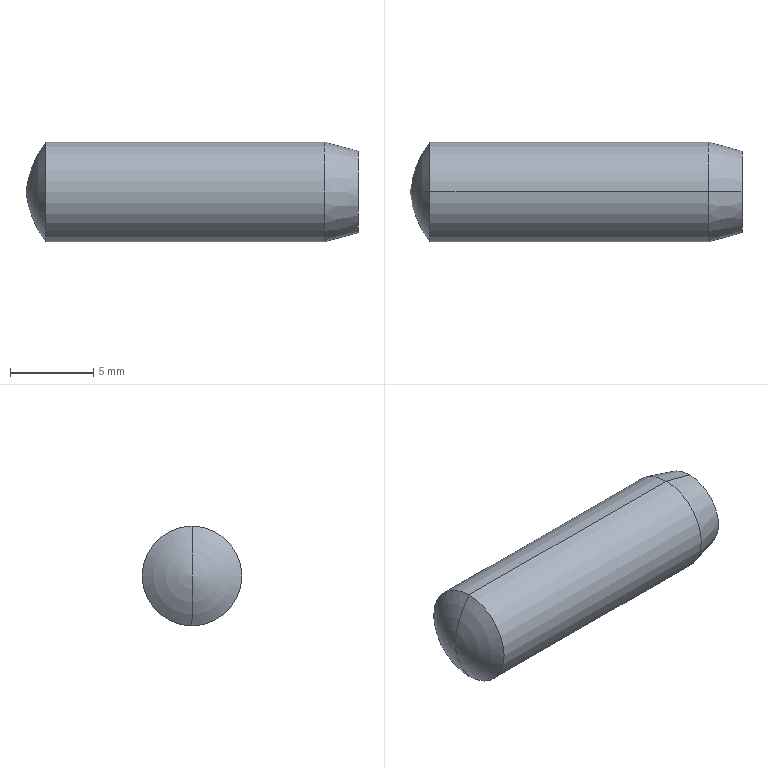Part | SolidWorks | features RefAxis 3, 3DProfileFeature 1, RevCut 1, Revolution 1 | 1 solid | 9 faces | box 20 x 6 x 6 mm | volume 537.381 mm3 | cone 4 | cylinder 2 | torus 2 | plane 1 | commonest cylinder face diameters 6 x2
STEP:
#1=CARTESIAN_POINT('',(8.,0.,0.));
#2=VERTEX_POINT('',#1);
#3=CARTESIAN_POINT('',(10.,0.,-0.5359));
#4=VERTEX_POINT('',#3);
#5=CARTESIAN_POINT('',(12.,0.,-1.072));
#6=DIRECTION('',(0.9659,0.,-0.2588));
#7=VECTOR('',#6,1000.);
#8=LINE('',#5,#7);
#9=EDGE_CURVE('',#2,#4,#8,.T.);
#10=ORIENTED_EDGE('',*,*,#9,.F.);
#11=CARTESIAN_POINT('',(10.,0.,0.5359));
#12=VERTEX_POINT('',#11);
#13=CARTESIAN_POINT('',(12.,0.,1.072));
#14=DIRECTION('',(0.9659,0.,0.2588));
#15=VECTOR('',#14,1000.);
#16=LINE('',#13,#15);
#17=EDGE_CURVE('',#2,#12,#16,.T.);
#18=ORIENTED_EDGE('',*,*,#17,.T.);
#19=CARTESIAN_POINT('',(10.,0.,0.));
#20=DIRECTION('',(1.,0.,0.));
#21=DIRECTION('',(0.,0.,1.));
#22=AXIS2_PLACEMENT_3D('',#19,#20,#21);
#23=CIRCLE('',#22,0.5359);
#24=EDGE_CURVE('',#12,#4,#23,.T.);
#25=ORIENTED_EDGE('',*,*,#24,.T.);
#26=EDGE_LOOP('',(#10,#18,#25));
#27=FACE_OUTER_BOUND('',#26,.T.);
#28=CARTESIAN_POINT('',(12.,0.,0.));
#29=DIRECTION('',(1.,0.,0.));
#30=DIRECTION('',(0.,0.,-1.));
#31=AXIS2_PLACEMENT_3D('',#28,#29,#30);
#32=CONICAL_SURFACE('',#31,1.072,0.2618);
#33=ADVANCED_FACE('',(#27),#32,.F.);
#34=CARTESIAN_POINT('',(10.,0.,2.464));
#35=VERTEX_POINT('',#34);
#36=CARTESIAN_POINT('',(10.,0.,-2.464));
#37=VERTEX_POINT('',#36);
#38=CARTESIAN_POINT('',(10.,0.,0.));
#39=DIRECTION('',(-1.,0.,0.));
#40=DIRECTION('',(0.,0.,1.));
#41=AXIS2_PLACEMENT_3D('',#38,#39,#40);
#42=CIRCLE('',#41,2.464);
#43=EDGE_CURVE('',#35,#37,#42,.T.);
#44=ORIENTED_EDGE('',*,*,#43,.T.);
#45=CARTESIAN_POINT('',(8.,0.,-3.));
#46=VERTEX_POINT('',#45);
#47=CARTESIAN_POINT('',(10.,0.,-2.464));
#48=DIRECTION('',(-0.9659,0.,-0.2588));
#49=VECTOR('',#48,1000.);
#50=LINE('',#47,#49);
#51=EDGE_CURVE('',#37,#46,#50,.T.);
#52=ORIENTED_EDGE('',*,*,#51,.T.);
#53=CARTESIAN_POINT('',(8.,0.,3.));
#54=VERTEX_POINT('',#53);
#55=CARTESIAN_POINT('',(8.,0.,0.));
#56=DIRECTION('',(-1.,0.,0.));
#57=DIRECTION('',(0.,0.,1.));
#58=AXIS2_PLACEMENT_3D('',#55,#56,#57);
#59=CIRCLE('',#58,3.);
#60=EDGE_CURVE('',#54,#46,#59,.T.);
#61=ORIENTED_EDGE('',*,*,#60,.F.);
#62=CARTESIAN_POINT('',(10.,0.,2.464));
#63=DIRECTION('',(-0.9659,0.,0.2588));
#64=VECTOR('',#63,1000.);
#65=LINE('',#62,#64);
#66=EDGE_CURVE('',#35,#54,#65,.T.);
#67=ORIENTED_EDGE('',*,*,#66,.F.);
#68=EDGE_LOOP('',(#44,#52,#61,#67));
#69=FACE_OUTER_BOUND('',#68,.T.);
#70=CARTESIAN_POINT('',(10.,0.,0.));
#71=DIRECTION('',(-1.,0.,0.));
#72=DIRECTION('',(0.,0.,1.));
#73=AXIS2_PLACEMENT_3D('',#70,#71,#72);
#74=CONICAL_SURFACE('',#73,2.464,0.2618);
#75=ADVANCED_FACE('',(#69),#74,.T.);
#76=ORIENTED_EDGE('',*,*,#60,.T.);
#77=CARTESIAN_POINT('',(-8.8,0.,-3.));
#78=VERTEX_POINT('',#77);
#79=CARTESIAN_POINT('',(10.,0.,-3.));
#80=DIRECTION('',(-1.,0.,0.));
#81=VECTOR('',#80,1000.);
#82=LINE('',#79,#81);
#83=EDGE_CURVE('',#46,#78,#82,.T.);
#84=ORIENTED_EDGE('',*,*,#83,.T.);
#85=CARTESIAN_POINT('',(-8.8,0.,3.));
#86=VERTEX_POINT('',#85);
#87=CARTESIAN_POINT('',(-8.8,0.,0.));
#88=DIRECTION('',(-1.,0.,0.));
#89=DIRECTION('',(0.,0.,1.));
#90=AXIS2_PLACEMENT_3D('',#87,#88,#89);
#91=CIRCLE('',#90,3.);
#92=EDGE_CURVE('',#86,#78,#91,.T.);
#93=ORIENTED_EDGE('',*,*,#92,.F.);
#94=CARTESIAN_POINT('',(10.,0.,3.));
#95=DIRECTION('',(-1.,0.,0.));
#96=VECTOR('',#95,1000.);
#97=LINE('',#94,#96);
#98=EDGE_CURVE('',#54,#86,#97,.T.);
#99=ORIENTED_EDGE('',*,*,#98,.F.);
#100=EDGE_LOOP('',(#76,#84,#93,#99));
#101=FACE_OUTER_BOUND('',#100,.T.);
#102=CARTESIAN_POINT('',(10.,0.,0.));
#103=DIRECTION('',(-1.,0.,0.));
#104=DIRECTION('',(0.,0.,1.));
#105=AXIS2_PLACEMENT_3D('',#102,#103,#104);
#106=CYLINDRICAL_SURFACE('',#105,3.);
#107=ADVANCED_FACE('',(#101),#106,.T.);
#108=ORIENTED_EDGE('',*,*,#92,.T.);
#109=CARTESIAN_POINT('',(-10.,0.,0.));
#110=VERTEX_POINT('',#109);
#111=CARTESIAN_POINT('',(-4.035,0.,0.646));
#112=DIRECTION('',(0.,1.,0.));
#113=DIRECTION('',(0.,0.,1.));
#114=AXIS2_PLACEMENT_3D('',#111,#112,#113);
#115=CIRCLE('',#114,6.);
#116=EDGE_CURVE('',#78,#110,#115,.T.);
#117=ORIENTED_EDGE('',*,*,#116,.T.);
#118=CARTESIAN_POINT('',(-4.035,0.,-0.646));
#119=DIRECTION('',(0.,-1.,0.));
#120=DIRECTION('',(0.,0.,-1.));
#121=AXIS2_PLACEMENT_3D('',#118,#119,#120);
#122=CIRCLE('',#121,6.);
#123=EDGE_CURVE('',#86,#110,#122,.T.);
#124=ORIENTED_EDGE('',*,*,#123,.F.);
#125=EDGE_LOOP('',(#108,#117,#124));
#126=FACE_OUTER_BOUND('',#125,.T.);
#127=CARTESIAN_POINT('',(-4.035,0.,0.));
#128=DIRECTION('',(-1.,0.,0.));
#129=DIRECTION('',(0.,0.,1.));
#130=AXIS2_PLACEMENT_3D('',#127,#128,#129);
#131=TOROIDAL_SURFACE('',#130,-0.646,6.);
#132=ADVANCED_FACE('',(#126),#131,.T.);
#133=ORIENTED_EDGE('',*,*,#43,.F.);
#134=CARTESIAN_POINT('',(10.,0.,0.));
#135=DIRECTION('',(-1.,0.,0.));
#136=DIRECTION('',(0.,0.,1.));
#137=AXIS2_PLACEMENT_3D('',#134,#135,#136);
#138=CIRCLE('',#137,2.464);
#139=EDGE_CURVE('',#37,#35,#138,.T.);
#140=ORIENTED_EDGE('',*,*,#139,.F.);
#141=EDGE_LOOP('',(#133,#140));
#142=FACE_OUTER_BOUND('',#141,.T.);
#143=CARTESIAN_POINT('',(10.,0.,0.));
#144=DIRECTION('',(1.,0.,0.));
#145=DIRECTION('',(0.,0.,1.));
#146=AXIS2_PLACEMENT_3D('',#143,#144,#145);
#147=CIRCLE('',#146,0.5359);
#148=EDGE_CURVE('',#4,#12,#147,.T.);
#149=ORIENTED_EDGE('',*,*,#148,.F.);
#150=ORIENTED_EDGE('',*,*,#24,.F.);
#151=EDGE_LOOP('',(#149,#150));
#152=FACE_BOUND('',#151,.T.);
#153=CARTESIAN_POINT('',(10.,2.464,0.));
#154=DIRECTION('',(-1.,0.,0.));
#155=DIRECTION('',(0.,0.,1.));
#156=AXIS2_PLACEMENT_3D('',#153,#154,#155);
#157=PLANE('',#156);
#158=ADVANCED_FACE('',(#142,#152),#157,.F.);
#159=ORIENTED_EDGE('',*,*,#116,.F.);
#160=CARTESIAN_POINT('',(-8.8,0.,0.));
#161=DIRECTION('',(-1.,0.,0.));
#162=DIRECTION('',(0.,0.,1.));
#163=AXIS2_PLACEMENT_3D('',#160,#161,#162);
#164=CIRCLE('',#163,3.);
#165=EDGE_CURVE('',#78,#86,#164,.T.);
#166=ORIENTED_EDGE('',*,*,#165,.T.);
#167=ORIENTED_EDGE('',*,*,#123,.T.);
#168=EDGE_LOOP('',(#159,#166,#167));
#169=FACE_OUTER_BOUND('',#168,.T.);
#170=CARTESIAN_POINT('',(-4.035,0.,0.));
#171=DIRECTION('',(-1.,0.,0.));
#172=DIRECTION('',(0.,0.,1.));
#173=AXIS2_PLACEMENT_3D('',#170,#171,#172);
#174=TOROIDAL_SURFACE('',#173,-0.646,6.);
#175=ADVANCED_FACE('',(#169),#174,.T.);
#176=ORIENTED_EDGE('',*,*,#83,.F.);
#177=CARTESIAN_POINT('',(8.,0.,0.));
#178=DIRECTION('',(-1.,0.,0.));
#179=DIRECTION('',(0.,0.,1.));
#180=AXIS2_PLACEMENT_3D('',#177,#178,#179);
#181=CIRCLE('',#180,3.);
#182=EDGE_CURVE('',#46,#54,#181,.T.);
#183=ORIENTED_EDGE('',*,*,#182,.T.);
#184=ORIENTED_EDGE('',*,*,#98,.T.);
#185=ORIENTED_EDGE('',*,*,#165,.F.);
#186=EDGE_LOOP('',(#176,#183,#184,#185));
#187=FACE_OUTER_BOUND('',#186,.T.);
#188=CARTESIAN_POINT('',(10.,0.,0.));
#189=DIRECTION('',(-1.,0.,0.));
#190=DIRECTION('',(0.,0.,1.));
#191=AXIS2_PLACEMENT_3D('',#188,#189,#190);
#192=CYLINDRICAL_SURFACE('',#191,3.);
#193=ADVANCED_FACE('',(#187),#192,.T.);
#194=ORIENTED_EDGE('',*,*,#51,.F.);
#195=ORIENTED_EDGE('',*,*,#139,.T.);
#196=ORIENTED_EDGE('',*,*,#66,.T.);
#197=ORIENTED_EDGE('',*,*,#182,.F.);
#198=EDGE_LOOP('',(#194,#195,#196,#197));
#199=FACE_OUTER_BOUND('',#198,.T.);
#200=CARTESIAN_POINT('',(10.,0.,0.));
#201=DIRECTION('',(-1.,0.,0.));
#202=DIRECTION('',(0.,0.,1.));
#203=AXIS2_PLACEMENT_3D('',#200,#201,#202);
#204=CONICAL_SURFACE('',#203,2.464,0.2618);
#205=ADVANCED_FACE('',(#199),#204,.T.);
#206=ORIENTED_EDGE('',*,*,#17,.F.);
#207=ORIENTED_EDGE('',*,*,#9,.T.);
#208=ORIENTED_EDGE('',*,*,#148,.T.);
#209=EDGE_LOOP('',(#206,#207,#208));
#210=FACE_OUTER_BOUND('',#209,.T.);
#211=CARTESIAN_POINT('',(12.,0.,0.));
#212=DIRECTION('',(1.,0.,0.));
#213=DIRECTION('',(0.,0.,-1.));
#214=AXIS2_PLACEMENT_3D('',#211,#212,#213);
#215=CONICAL_SURFACE('',#214,1.072,0.2618);
#216=ADVANCED_FACE('',(#210),#215,.F.);
#217=CLOSED_SHELL('',(#33,#75,#107,#132,#158,#175,#193,#205,#216));
#218=MANIFOLD_SOLID_BREP('',#217);
#219=CARTESIAN_POINT('',(0.,0.,0.));
#220=DIRECTION('',(0.,0.,1.));
#221=DIRECTION('',(1.,0.,0.));
#222=AXIS2_PLACEMENT_3D('',#219,#220,#221);
#223=(LENGTH_UNIT()NAMED_UNIT(*)SI_UNIT(.MILLI.,.METRE.));
#224=UNCERTAINTY_MEASURE_WITH_UNIT(LENGTH_MEASURE(0.00001),#223,'','');
#225=(NAMED_UNIT(*)PLANE_ANGLE_UNIT()SI_UNIT($,.RADIAN.));
#226=(NAMED_UNIT(*)SI_UNIT($,.STERADIAN.)SOLID_ANGLE_UNIT());
#227=(GEOMETRIC_REPRESENTATION_CONTEXT(3)GLOBAL_UNCERTAINTY_ASSIGNED_CONTEXT((#224))GLOBAL_UNIT_ASSIGNED_CONTEXT((#223,#225,#226))REPRESENTATION_CONTEXT('',''));
#228=ADVANCED_BREP_SHAPE_REPRESENTATION('',(#218,#222),#227);